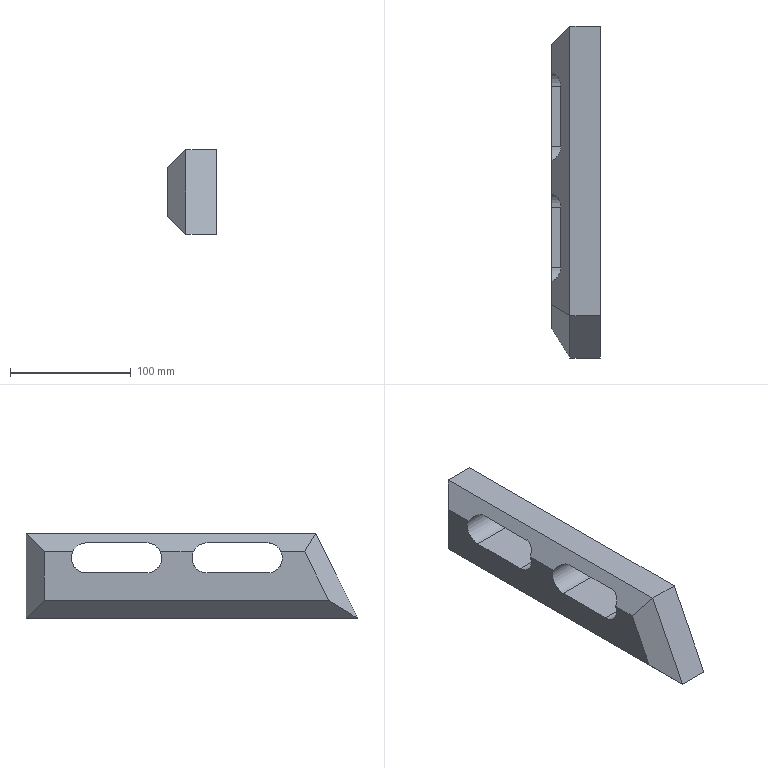Part | SolidWorks | features Chamfer 1, Extrusion 1 | 1 solid | 18 faces | box 40 x 275 x 70 mm | volume 515457 mm3 | plane 14 | cylinder 4 | commonest cylinder face diameters 25 x4
STEP:
#1=CARTESIAN_POINT('',(20.,140.,-7.5));
#2=VERTEX_POINT('',#1);
#3=CARTESIAN_POINT('',(20.,140.,-32.5));
#4=VERTEX_POINT('',#3);
#5=CARTESIAN_POINT('',(20.,140.,-20.));
#6=DIRECTION('',(1.,0.,0.));
#7=DIRECTION('',(0.,0.,-1.));
#8=AXIS2_PLACEMENT_3D('',#5,#6,#7);
#9=CIRCLE('',#8,12.5);
#10=EDGE_CURVE('',#2,#4,#9,.T.);
#11=ORIENTED_EDGE('',*,*,#10,.F.);
#12=CARTESIAN_POINT('',(20.,190.,-7.5));
#13=VERTEX_POINT('',#12);
#14=CARTESIAN_POINT('',(20.,140.,-7.5));
#15=DIRECTION('',(0.,-1.,0.));
#16=VECTOR('',#15,1000.);
#17=LINE('',#14,#16);
#18=EDGE_CURVE('',#13,#2,#17,.T.);
#19=ORIENTED_EDGE('',*,*,#18,.F.);
#20=CARTESIAN_POINT('',(20.,190.,-32.5));
#21=VERTEX_POINT('',#20);
#22=CARTESIAN_POINT('',(20.,190.,-20.));
#23=DIRECTION('',(1.,0.,0.));
#24=DIRECTION('',(0.,0.,-1.));
#25=AXIS2_PLACEMENT_3D('',#22,#23,#24);
#26=CIRCLE('',#25,12.5);
#27=EDGE_CURVE('',#21,#13,#26,.T.);
#28=ORIENTED_EDGE('',*,*,#27,.F.);
#29=CARTESIAN_POINT('',(20.,140.,-32.5));
#30=DIRECTION('',(0.,1.,0.));
#31=VECTOR('',#30,1000.);
#32=LINE('',#29,#31);
#33=EDGE_CURVE('',#4,#21,#32,.T.);
#34=ORIENTED_EDGE('',*,*,#33,.F.);
#35=EDGE_LOOP('',(#11,#19,#28,#34));
#36=FACE_BOUND('',#35,.T.);
#37=CARTESIAN_POINT('',(20.,240.,0.));
#38=VERTEX_POINT('',#37);
#39=CARTESIAN_POINT('',(20.,0.,0.));
#40=VERTEX_POINT('',#39);
#41=CARTESIAN_POINT('',(20.,240.,0.));
#42=DIRECTION('',(0.,-1.,0.));
#43=VECTOR('',#42,1000.);
#44=LINE('',#41,#43);
#45=EDGE_CURVE('',#38,#40,#44,.T.);
#46=ORIENTED_EDGE('',*,*,#45,.T.);
#47=CARTESIAN_POINT('',(20.,-35.,-70.));
#48=VERTEX_POINT('',#47);
#49=CARTESIAN_POINT('',(20.,0.,0.));
#50=DIRECTION('',(0.,-0.4472,-0.8944));
#51=VECTOR('',#50,1000.);
#52=LINE('',#49,#51);
#53=EDGE_CURVE('',#40,#48,#52,.T.);
#54=ORIENTED_EDGE('',*,*,#53,.T.);
#55=CARTESIAN_POINT('',(20.,240.,-70.));
#56=VERTEX_POINT('',#55);
#57=CARTESIAN_POINT('',(20.,-35.,-70.));
#58=DIRECTION('',(0.,1.,0.));
#59=VECTOR('',#58,1000.);
#60=LINE('',#57,#59);
#61=EDGE_CURVE('',#48,#56,#60,.T.);
#62=ORIENTED_EDGE('',*,*,#61,.T.);
#63=CARTESIAN_POINT('',(20.,240.,-70.));
#64=DIRECTION('',(0.,0.,1.));
#65=VECTOR('',#64,1000.);
#66=LINE('',#63,#65);
#67=EDGE_CURVE('',#56,#38,#66,.T.);
#68=ORIENTED_EDGE('',*,*,#67,.T.);
#69=EDGE_LOOP('',(#46,#54,#62,#68));
#70=FACE_OUTER_BOUND('',#69,.T.);
#71=CARTESIAN_POINT('',(20.,40.,-7.5));
#72=VERTEX_POINT('',#71);
#73=CARTESIAN_POINT('',(20.,40.,-32.5));
#74=VERTEX_POINT('',#73);
#75=CARTESIAN_POINT('',(20.,40.,-20.));
#76=DIRECTION('',(1.,0.,0.));
#77=DIRECTION('',(0.,0.,-1.));
#78=AXIS2_PLACEMENT_3D('',#75,#76,#77);
#79=CIRCLE('',#78,12.5);
#80=EDGE_CURVE('',#72,#74,#79,.T.);
#81=ORIENTED_EDGE('',*,*,#80,.F.);
#82=CARTESIAN_POINT('',(20.,90.,-7.5));
#83=VERTEX_POINT('',#82);
#84=CARTESIAN_POINT('',(20.,40.,-7.5));
#85=DIRECTION('',(0.,-1.,0.));
#86=VECTOR('',#85,1000.);
#87=LINE('',#84,#86);
#88=EDGE_CURVE('',#83,#72,#87,.T.);
#89=ORIENTED_EDGE('',*,*,#88,.F.);
#90=CARTESIAN_POINT('',(20.,90.,-32.5));
#91=VERTEX_POINT('',#90);
#92=CARTESIAN_POINT('',(20.,90.,-20.));
#93=DIRECTION('',(1.,0.,0.));
#94=DIRECTION('',(0.,0.,-1.));
#95=AXIS2_PLACEMENT_3D('',#92,#93,#94);
#96=CIRCLE('',#95,12.5);
#97=EDGE_CURVE('',#91,#83,#96,.T.);
#98=ORIENTED_EDGE('',*,*,#97,.F.);
#99=CARTESIAN_POINT('',(20.,40.,-32.5));
#100=DIRECTION('',(0.,1.,0.));
#101=VECTOR('',#100,1000.);
#102=LINE('',#99,#101);
#103=EDGE_CURVE('',#74,#91,#102,.T.);
#104=ORIENTED_EDGE('',*,*,#103,.F.);
#105=EDGE_LOOP('',(#81,#89,#98,#104));
#106=FACE_BOUND('',#105,.T.);
#107=CARTESIAN_POINT('',(20.,0.,0.));
#108=DIRECTION('',(-1.,0.,0.));
#109=DIRECTION('',(0.,0.,1.));
#110=AXIS2_PLACEMENT_3D('',#107,#108,#109);
#111=PLANE('',#110);
#112=ADVANCED_FACE('',(#36,#70,#106),#111,.F.);
#113=CARTESIAN_POINT('',(-20.,90.,-32.5));
#114=VERTEX_POINT('',#113);
#115=CARTESIAN_POINT('',(-20.,101.456,-15.));
#116=VERTEX_POINT('',#115);
#117=CARTESIAN_POINT('',(-20.,90.,-20.));
#118=DIRECTION('',(1.,0.,0.));
#119=DIRECTION('',(0.,0.,-1.));
#120=AXIS2_PLACEMENT_3D('',#117,#118,#119);
#121=CIRCLE('',#120,12.5);
#122=EDGE_CURVE('',#114,#116,#121,.T.);
#123=ORIENTED_EDGE('',*,*,#122,.T.);
#124=CARTESIAN_POINT('',(-20.,128.544,-15.));
#125=VERTEX_POINT('',#124);
#126=CARTESIAN_POINT('',(-20.,240.,-15.));
#127=DIRECTION('',(0.,1.,0.));
#128=VECTOR('',#127,1000.);
#129=LINE('',#126,#128);
#130=EDGE_CURVE('',#116,#125,#129,.T.);
#131=ORIENTED_EDGE('',*,*,#130,.T.);
#132=CARTESIAN_POINT('',(-20.,140.,-32.5));
#133=VERTEX_POINT('',#132);
#134=CARTESIAN_POINT('',(-20.,140.,-20.));
#135=DIRECTION('',(1.,0.,0.));
#136=DIRECTION('',(0.,0.,-1.));
#137=AXIS2_PLACEMENT_3D('',#134,#135,#136);
#138=CIRCLE('',#137,12.5);
#139=EDGE_CURVE('',#125,#133,#138,.T.);
#140=ORIENTED_EDGE('',*,*,#139,.T.);
#141=CARTESIAN_POINT('',(-20.,190.,-32.5));
#142=VERTEX_POINT('',#141);
#143=CARTESIAN_POINT('',(-20.,140.,-32.5));
#144=DIRECTION('',(0.,1.,0.));
#145=VECTOR('',#144,1000.);
#146=LINE('',#143,#145);
#147=EDGE_CURVE('',#133,#142,#146,.T.);
#148=ORIENTED_EDGE('',*,*,#147,.T.);
#149=CARTESIAN_POINT('',(-20.,201.456,-15.));
#150=VERTEX_POINT('',#149);
#151=CARTESIAN_POINT('',(-20.,190.,-20.));
#152=DIRECTION('',(1.,0.,0.));
#153=DIRECTION('',(0.,0.,-1.));
#154=AXIS2_PLACEMENT_3D('',#151,#152,#153);
#155=CIRCLE('',#154,12.5);
#156=EDGE_CURVE('',#142,#150,#155,.T.);
#157=ORIENTED_EDGE('',*,*,#156,.T.);
#158=CARTESIAN_POINT('',(-20.,225.,-15.));
#159=VERTEX_POINT('',#158);
#160=CARTESIAN_POINT('',(-20.,240.,-15.));
#161=DIRECTION('',(0.,1.,0.));
#162=VECTOR('',#161,1000.);
#163=LINE('',#160,#162);
#164=EDGE_CURVE('',#150,#159,#163,.T.);
#165=ORIENTED_EDGE('',*,*,#164,.T.);
#166=CARTESIAN_POINT('',(-20.,225.,-55.));
#167=VERTEX_POINT('',#166);
#168=CARTESIAN_POINT('',(-20.,225.,-70.));
#169=DIRECTION('',(0.,0.,-1.));
#170=VECTOR('',#169,1000.);
#171=LINE('',#168,#170);
#172=EDGE_CURVE('',#159,#167,#171,.T.);
#173=ORIENTED_EDGE('',*,*,#172,.T.);
#174=CARTESIAN_POINT('',(-20.,-10.729,-55.));
#175=VERTEX_POINT('',#174);
#176=CARTESIAN_POINT('',(-20.,-35.,-55.));
#177=DIRECTION('',(0.,-1.,0.));
#178=VECTOR('',#177,1000.);
#179=LINE('',#176,#178);
#180=EDGE_CURVE('',#167,#175,#179,.T.);
#181=ORIENTED_EDGE('',*,*,#180,.T.);
#182=CARTESIAN_POINT('',(-20.,9.271,-15.));
#183=VERTEX_POINT('',#182);
#184=CARTESIAN_POINT('',(-20.,13.416,-6.708));
#185=DIRECTION('',(0.,0.4472,0.8944));
#186=VECTOR('',#185,1000.);
#187=LINE('',#184,#186);
#188=EDGE_CURVE('',#175,#183,#187,.T.);
#189=ORIENTED_EDGE('',*,*,#188,.T.);
#190=CARTESIAN_POINT('',(-20.,28.544,-15.));
#191=VERTEX_POINT('',#190);
#192=CARTESIAN_POINT('',(-20.,240.,-15.));
#193=DIRECTION('',(0.,1.,0.));
#194=VECTOR('',#193,1000.);
#195=LINE('',#192,#194);
#196=EDGE_CURVE('',#183,#191,#195,.T.);
#197=ORIENTED_EDGE('',*,*,#196,.T.);
#198=CARTESIAN_POINT('',(-20.,40.,-32.5));
#199=VERTEX_POINT('',#198);
#200=CARTESIAN_POINT('',(-20.,40.,-20.));
#201=DIRECTION('',(1.,0.,0.));
#202=DIRECTION('',(0.,0.,-1.));
#203=AXIS2_PLACEMENT_3D('',#200,#201,#202);
#204=CIRCLE('',#203,12.5);
#205=EDGE_CURVE('',#191,#199,#204,.T.);
#206=ORIENTED_EDGE('',*,*,#205,.T.);
#207=CARTESIAN_POINT('',(-20.,40.,-32.5));
#208=DIRECTION('',(0.,1.,0.));
#209=VECTOR('',#208,1000.);
#210=LINE('',#207,#209);
#211=EDGE_CURVE('',#199,#114,#210,.T.);
#212=ORIENTED_EDGE('',*,*,#211,.T.);
#213=EDGE_LOOP('',(#123,#131,#140,#148,#157,#165,#173,#181,#189,#197,#206,#212));
#214=FACE_OUTER_BOUND('',#213,.T.);
#215=CARTESIAN_POINT('',(-20.,0.,0.));
#216=DIRECTION('',(-1.,0.,0.));
#217=DIRECTION('',(0.,0.,1.));
#218=AXIS2_PLACEMENT_3D('',#215,#216,#217);
#219=PLANE('',#218);
#220=ADVANCED_FACE('',(#214),#219,.T.);
#221=CARTESIAN_POINT('',(-5.,240.,0.));
#222=VERTEX_POINT('',#221);
#223=CARTESIAN_POINT('',(20.,240.,0.));
#224=DIRECTION('',(-1.,0.,0.));
#225=VECTOR('',#224,1000.);
#226=LINE('',#223,#225);
#227=EDGE_CURVE('',#38,#222,#226,.T.);
#228=ORIENTED_EDGE('',*,*,#227,.T.);
#229=CARTESIAN_POINT('',(-5.,0.,0.));
#230=VERTEX_POINT('',#229);
#231=CARTESIAN_POINT('',(-5.,0.,0.));
#232=DIRECTION('',(0.,-1.,0.));
#233=VECTOR('',#232,1000.);
#234=LINE('',#231,#233);
#235=EDGE_CURVE('',#222,#230,#234,.T.);
#236=ORIENTED_EDGE('',*,*,#235,.T.);
#237=CARTESIAN_POINT('',(20.,0.,0.));
#238=DIRECTION('',(-1.,0.,0.));
#239=VECTOR('',#238,1000.);
#240=LINE('',#237,#239);
#241=EDGE_CURVE('',#40,#230,#240,.T.);
#242=ORIENTED_EDGE('',*,*,#241,.F.);
#243=ORIENTED_EDGE('',*,*,#45,.F.);
#244=EDGE_LOOP('',(#228,#236,#242,#243));
#245=FACE_OUTER_BOUND('',#244,.T.);
#246=CARTESIAN_POINT('',(20.,240.,0.));
#247=DIRECTION('',(0.,0.,-1.));
#248=DIRECTION('',(-1.,0.,0.));
#249=AXIS2_PLACEMENT_3D('',#246,#247,#248);
#250=PLANE('',#249);
#251=ADVANCED_FACE('',(#245),#250,.F.);
#252=ORIENTED_EDGE('',*,*,#241,.T.);
#253=CARTESIAN_POINT('',(-5.,-35.,-70.));
#254=VERTEX_POINT('',#253);
#255=CARTESIAN_POINT('',(-5.,-35.,-70.));
#256=DIRECTION('',(0.,-0.4472,-0.8944));
#257=VECTOR('',#256,1000.);
#258=LINE('',#255,#257);
#259=EDGE_CURVE('',#230,#254,#258,.T.);
#260=ORIENTED_EDGE('',*,*,#259,.T.);
#261=CARTESIAN_POINT('',(20.,-35.,-70.));
#262=DIRECTION('',(-1.,0.,0.));
#263=VECTOR('',#262,1000.);
#264=LINE('',#261,#263);
#265=EDGE_CURVE('',#48,#254,#264,.T.);
#266=ORIENTED_EDGE('',*,*,#265,.F.);
#267=ORIENTED_EDGE('',*,*,#53,.F.);
#268=EDGE_LOOP('',(#252,#260,#266,#267));
#269=FACE_OUTER_BOUND('',#268,.T.);
#270=CARTESIAN_POINT('',(20.,0.,0.));
#271=DIRECTION('',(0.,0.8944,-0.4472));
#272=DIRECTION('',(0.,0.4472,0.8944));
#273=AXIS2_PLACEMENT_3D('',#270,#271,#272);
#274=PLANE('',#273);
#275=ADVANCED_FACE('',(#269),#274,.F.);
#276=ORIENTED_EDGE('',*,*,#265,.T.);
#277=CARTESIAN_POINT('',(-5.,240.,-70.));
#278=VERTEX_POINT('',#277);
#279=CARTESIAN_POINT('',(-5.,240.,-70.));
#280=DIRECTION('',(0.,1.,0.));
#281=VECTOR('',#280,1000.);
#282=LINE('',#279,#281);
#283=EDGE_CURVE('',#254,#278,#282,.T.);
#284=ORIENTED_EDGE('',*,*,#283,.T.);
#285=CARTESIAN_POINT('',(20.,240.,-70.));
#286=DIRECTION('',(-1.,0.,0.));
#287=VECTOR('',#286,1000.);
#288=LINE('',#285,#287);
#289=EDGE_CURVE('',#56,#278,#288,.T.);
#290=ORIENTED_EDGE('',*,*,#289,.F.);
#291=ORIENTED_EDGE('',*,*,#61,.F.);
#292=EDGE_LOOP('',(#276,#284,#290,#291));
#293=FACE_OUTER_BOUND('',#292,.T.);
#294=CARTESIAN_POINT('',(20.,-35.,-70.));
#295=DIRECTION('',(0.,0.,1.));
#296=DIRECTION('',(0.,-1.,0.));
#297=AXIS2_PLACEMENT_3D('',#294,#295,#296);
#298=PLANE('',#297);
#299=ADVANCED_FACE('',(#293),#298,.F.);
#300=ORIENTED_EDGE('',*,*,#289,.T.);
#301=CARTESIAN_POINT('',(-5.,240.,0.));
#302=DIRECTION('',(0.,0.,1.));
#303=VECTOR('',#302,1000.);
#304=LINE('',#301,#303);
#305=EDGE_CURVE('',#278,#222,#304,.T.);
#306=ORIENTED_EDGE('',*,*,#305,.T.);
#307=ORIENTED_EDGE('',*,*,#227,.F.);
#308=ORIENTED_EDGE('',*,*,#67,.F.);
#309=EDGE_LOOP('',(#300,#306,#307,#308));
#310=FACE_OUTER_BOUND('',#309,.T.);
#311=CARTESIAN_POINT('',(20.,240.,-70.));
#312=DIRECTION('',(0.,-1.,0.));
#313=DIRECTION('',(0.,0.,-1.));
#314=AXIS2_PLACEMENT_3D('',#311,#312,#313);
#315=PLANE('',#314);
#316=ADVANCED_FACE('',(#310),#315,.F.);
#317=ORIENTED_EDGE('',*,*,#139,.F.);
#318=CARTESIAN_POINT('',(-12.5,140.,-7.5));
#319=VERTEX_POINT('',#318);
#320=CARTESIAN_POINT('',(-20.,128.544,-15.));
#321=CARTESIAN_POINT('',(-15.306,130.592,-10.306));
#322=CARTESIAN_POINT('',(-12.5,134.878,-7.5));
#323=CARTESIAN_POINT('',(-12.5,140.,-7.5));
#324=(BOUNDED_CURVE()B_SPLINE_CURVE(3,(#320,#321,#322,#323),.UNSPECIFIED.,.F.,.T.)B_SPLINE_CURVE_WITH_KNOTS((4,4),(1.982,3.142),.UNSPECIFIED.)CURVE()GEOMETRIC_REPRESENTATION_ITEM()RATIONAL_B_SPLINE_CURVE((1.,0.8911,0.8911,1.))REPRESENTATION_ITEM(''));
#325=EDGE_CURVE('',#125,#319,#324,.T.);
#326=ORIENTED_EDGE('',*,*,#325,.T.);
#327=CARTESIAN_POINT('',(20.,140.,-7.5));
#328=DIRECTION('',(-1.,0.,0.));
#329=VECTOR('',#328,1000.);
#330=LINE('',#327,#329);
#331=EDGE_CURVE('',#2,#319,#330,.T.);
#332=ORIENTED_EDGE('',*,*,#331,.F.);
#333=ORIENTED_EDGE('',*,*,#10,.T.);
#334=CARTESIAN_POINT('',(20.,140.,-32.5));
#335=DIRECTION('',(-1.,0.,0.));
#336=VECTOR('',#335,1000.);
#337=LINE('',#334,#336);
#338=EDGE_CURVE('',#4,#133,#337,.T.);
#339=ORIENTED_EDGE('',*,*,#338,.T.);
#340=EDGE_LOOP('',(#317,#326,#332,#333,#339));
#341=FACE_OUTER_BOUND('',#340,.T.);
#342=CARTESIAN_POINT('',(20.,140.,-20.));
#343=DIRECTION('',(-1.,0.,0.));
#344=DIRECTION('',(0.,0.,1.));
#345=AXIS2_PLACEMENT_3D('',#342,#343,#344);
#346=CYLINDRICAL_SURFACE('',#345,12.5);
#347=ADVANCED_FACE('',(#341),#346,.F.);
#348=ORIENTED_EDGE('',*,*,#147,.F.);
#349=ORIENTED_EDGE('',*,*,#338,.F.);
#350=ORIENTED_EDGE('',*,*,#33,.T.);
#351=CARTESIAN_POINT('',(20.,190.,-32.5));
#352=DIRECTION('',(-1.,0.,0.));
#353=VECTOR('',#352,1000.);
#354=LINE('',#351,#353);
#355=EDGE_CURVE('',#21,#142,#354,.T.);
#356=ORIENTED_EDGE('',*,*,#355,.T.);
#357=EDGE_LOOP('',(#348,#349,#350,#356));
#358=FACE_OUTER_BOUND('',#357,.T.);
#359=CARTESIAN_POINT('',(20.,140.,-32.5));
#360=DIRECTION('',(0.,0.,1.));
#361=DIRECTION('',(1.,0.,0.));
#362=AXIS2_PLACEMENT_3D('',#359,#360,#361);
#363=PLANE('',#362);
#364=ADVANCED_FACE('',(#358),#363,.T.);
#365=CARTESIAN_POINT('',(-12.5,190.,-7.5));
#366=VERTEX_POINT('',#365);
#367=CARTESIAN_POINT('',(20.,190.,-7.5));
#368=DIRECTION('',(-1.,0.,0.));
#369=VECTOR('',#368,1000.);
#370=LINE('',#367,#369);
#371=EDGE_CURVE('',#13,#366,#370,.T.);
#372=ORIENTED_EDGE('',*,*,#371,.T.);
#373=CARTESIAN_POINT('',(-12.5,190.,-7.5));
#374=CARTESIAN_POINT('',(-12.5,195.122,-7.5));
#375=CARTESIAN_POINT('',(-15.306,199.408,-10.306));
#376=CARTESIAN_POINT('',(-20.,201.456,-15.));
#377=(BOUNDED_CURVE()B_SPLINE_CURVE(3,(#373,#374,#375,#376),.UNSPECIFIED.,.F.,.T.)B_SPLINE_CURVE_WITH_KNOTS((4,4),(3.142,4.301),.UNSPECIFIED.)CURVE()GEOMETRIC_REPRESENTATION_ITEM()RATIONAL_B_SPLINE_CURVE((1.,0.8911,0.8911,1.))REPRESENTATION_ITEM(''));
#378=EDGE_CURVE('',#366,#150,#377,.T.);
#379=ORIENTED_EDGE('',*,*,#378,.T.);
#380=ORIENTED_EDGE('',*,*,#156,.F.);
#381=ORIENTED_EDGE('',*,*,#355,.F.);
#382=ORIENTED_EDGE('',*,*,#27,.T.);
#383=EDGE_LOOP('',(#372,#379,#380,#381,#382));
#384=FACE_OUTER_BOUND('',#383,.T.);
#385=CARTESIAN_POINT('',(20.,190.,-20.));
#386=DIRECTION('',(-1.,0.,0.));
#387=DIRECTION('',(0.,0.,1.));
#388=AXIS2_PLACEMENT_3D('',#385,#386,#387);
#389=CYLINDRICAL_SURFACE('',#388,12.5);
#390=ADVANCED_FACE('',(#384),#389,.F.);
#391=ORIENTED_EDGE('',*,*,#331,.T.);
#392=CARTESIAN_POINT('',(-12.5,140.,-7.5));
#393=DIRECTION('',(0.,1.,0.));
#394=VECTOR('',#393,1000.);
#395=LINE('',#392,#394);
#396=EDGE_CURVE('',#319,#366,#395,.T.);
#397=ORIENTED_EDGE('',*,*,#396,.T.);
#398=ORIENTED_EDGE('',*,*,#371,.F.);
#399=ORIENTED_EDGE('',*,*,#18,.T.);
#400=EDGE_LOOP('',(#391,#397,#398,#399));
#401=FACE_OUTER_BOUND('',#400,.T.);
#402=CARTESIAN_POINT('',(20.,140.,-7.5));
#403=DIRECTION('',(0.,0.,-1.));
#404=DIRECTION('',(-1.,0.,0.));
#405=AXIS2_PLACEMENT_3D('',#402,#403,#404);
#406=PLANE('',#405);
#407=ADVANCED_FACE('',(#401),#406,.T.);
#408=ORIENTED_EDGE('',*,*,#205,.F.);
#409=CARTESIAN_POINT('',(-12.5,40.,-7.5));
#410=VERTEX_POINT('',#409);
#411=CARTESIAN_POINT('',(-20.,28.544,-15.));
#412=CARTESIAN_POINT('',(-15.306,30.592,-10.306));
#413=CARTESIAN_POINT('',(-12.5,34.878,-7.5));
#414=CARTESIAN_POINT('',(-12.5,40.,-7.5));
#415=(BOUNDED_CURVE()B_SPLINE_CURVE(3,(#411,#412,#413,#414),.UNSPECIFIED.,.F.,.T.)B_SPLINE_CURVE_WITH_KNOTS((4,4),(1.982,3.142),.UNSPECIFIED.)CURVE()GEOMETRIC_REPRESENTATION_ITEM()RATIONAL_B_SPLINE_CURVE((1.,0.8911,0.8911,1.))REPRESENTATION_ITEM(''));
#416=EDGE_CURVE('',#191,#410,#415,.T.);
#417=ORIENTED_EDGE('',*,*,#416,.T.);
#418=CARTESIAN_POINT('',(20.,40.,-7.5));
#419=DIRECTION('',(-1.,0.,0.));
#420=VECTOR('',#419,1000.);
#421=LINE('',#418,#420);
#422=EDGE_CURVE('',#72,#410,#421,.T.);
#423=ORIENTED_EDGE('',*,*,#422,.F.);
#424=ORIENTED_EDGE('',*,*,#80,.T.);
#425=CARTESIAN_POINT('',(20.,40.,-32.5));
#426=DIRECTION('',(-1.,0.,0.));
#427=VECTOR('',#426,1000.);
#428=LINE('',#425,#427);
#429=EDGE_CURVE('',#74,#199,#428,.T.);
#430=ORIENTED_EDGE('',*,*,#429,.T.);
#431=EDGE_LOOP('',(#408,#417,#423,#424,#430));
#432=FACE_OUTER_BOUND('',#431,.T.);
#433=CARTESIAN_POINT('',(20.,40.,-20.));
#434=DIRECTION('',(-1.,0.,0.));
#435=DIRECTION('',(0.,0.,1.));
#436=AXIS2_PLACEMENT_3D('',#433,#434,#435);
#437=CYLINDRICAL_SURFACE('',#436,12.5);
#438=ADVANCED_FACE('',(#432),#437,.F.);
#439=ORIENTED_EDGE('',*,*,#211,.F.);
#440=ORIENTED_EDGE('',*,*,#429,.F.);
#441=ORIENTED_EDGE('',*,*,#103,.T.);
#442=CARTESIAN_POINT('',(20.,90.,-32.5));
#443=DIRECTION('',(-1.,0.,0.));
#444=VECTOR('',#443,1000.);
#445=LINE('',#442,#444);
#446=EDGE_CURVE('',#91,#114,#445,.T.);
#447=ORIENTED_EDGE('',*,*,#446,.T.);
#448=EDGE_LOOP('',(#439,#440,#441,#447));
#449=FACE_OUTER_BOUND('',#448,.T.);
#450=CARTESIAN_POINT('',(20.,40.,-32.5));
#451=DIRECTION('',(0.,0.,1.));
#452=DIRECTION('',(1.,0.,0.));
#453=AXIS2_PLACEMENT_3D('',#450,#451,#452);
#454=PLANE('',#453);
#455=ADVANCED_FACE('',(#449),#454,.T.);
#456=CARTESIAN_POINT('',(-12.5,90.,-7.5));
#457=VERTEX_POINT('',#456);
#458=CARTESIAN_POINT('',(20.,90.,-7.5));
#459=DIRECTION('',(-1.,0.,0.));
#460=VECTOR('',#459,1000.);
#461=LINE('',#458,#460);
#462=EDGE_CURVE('',#83,#457,#461,.T.);
#463=ORIENTED_EDGE('',*,*,#462,.T.);
#464=CARTESIAN_POINT('',(-12.5,90.,-7.5));
#465=CARTESIAN_POINT('',(-12.5,95.122,-7.5));
#466=CARTESIAN_POINT('',(-15.306,99.408,-10.306));
#467=CARTESIAN_POINT('',(-20.,101.456,-15.));
#468=(BOUNDED_CURVE()B_SPLINE_CURVE(3,(#464,#465,#466,#467),.UNSPECIFIED.,.F.,.F.)B_SPLINE_CURVE_WITH_KNOTS((4,4),(3.142,4.301),.UNSPECIFIED.)CURVE()GEOMETRIC_REPRESENTATION_ITEM()RATIONAL_B_SPLINE_CURVE((1.,0.8911,0.8911,1.))REPRESENTATION_ITEM(''));
#469=EDGE_CURVE('',#457,#116,#468,.T.);
#470=ORIENTED_EDGE('',*,*,#469,.T.);
#471=ORIENTED_EDGE('',*,*,#122,.F.);
#472=ORIENTED_EDGE('',*,*,#446,.F.);
#473=ORIENTED_EDGE('',*,*,#97,.T.);
#474=EDGE_LOOP('',(#463,#470,#471,#472,#473));
#475=FACE_OUTER_BOUND('',#474,.T.);
#476=CARTESIAN_POINT('',(20.,90.,-20.));
#477=DIRECTION('',(-1.,0.,0.));
#478=DIRECTION('',(0.,0.,1.));
#479=AXIS2_PLACEMENT_3D('',#476,#477,#478);
#480=CYLINDRICAL_SURFACE('',#479,12.5);
#481=ADVANCED_FACE('',(#475),#480,.F.);
#482=ORIENTED_EDGE('',*,*,#422,.T.);
#483=CARTESIAN_POINT('',(-12.5,40.,-7.5));
#484=DIRECTION('',(0.,1.,0.));
#485=VECTOR('',#484,1000.);
#486=LINE('',#483,#485);
#487=EDGE_CURVE('',#410,#457,#486,.T.);
#488=ORIENTED_EDGE('',*,*,#487,.T.);
#489=ORIENTED_EDGE('',*,*,#462,.F.);
#490=ORIENTED_EDGE('',*,*,#88,.T.);
#491=EDGE_LOOP('',(#482,#488,#489,#490));
#492=FACE_OUTER_BOUND('',#491,.T.);
#493=CARTESIAN_POINT('',(20.,40.,-7.5));
#494=DIRECTION('',(0.,0.,-1.));
#495=DIRECTION('',(-1.,0.,0.));
#496=AXIS2_PLACEMENT_3D('',#493,#494,#495);
#497=PLANE('',#496);
#498=ADVANCED_FACE('',(#492),#497,.T.);
#499=CARTESIAN_POINT('',(-5.,240.,-70.));
#500=DIRECTION('',(0.5774,0.5774,-0.5774));
#501=VECTOR('',#500,1000.);
#502=LINE('',#499,#501);
#503=EDGE_CURVE('',#167,#278,#502,.T.);
#504=ORIENTED_EDGE('',*,*,#503,.F.);
#505=ORIENTED_EDGE('',*,*,#172,.F.);
#506=CARTESIAN_POINT('',(-28.333,216.667,-23.333));
#507=DIRECTION('',(-0.5774,-0.5774,-0.5774));
#508=VECTOR('',#507,1000.);
#509=LINE('',#506,#508);
#510=EDGE_CURVE('',#222,#159,#509,.T.);
#511=ORIENTED_EDGE('',*,*,#510,.F.);
#512=ORIENTED_EDGE('',*,*,#305,.F.);
#513=EDGE_LOOP('',(#504,#505,#511,#512));
#514=FACE_OUTER_BOUND('',#513,.T.);
#515=CARTESIAN_POINT('',(-5.,240.,-70.));
#516=DIRECTION('',(-0.7071,0.7071,0.));
#517=DIRECTION('',(0.,0.,-1.));
#518=AXIS2_PLACEMENT_3D('',#515,#516,#517);
#519=PLANE('',#518);
#520=ADVANCED_FACE('',(#514),#519,.T.);
#521=ORIENTED_EDGE('',*,*,#416,.F.);
#522=ORIENTED_EDGE('',*,*,#196,.F.);
#523=CARTESIAN_POINT('',(-67.271,38.486,-62.271));
#524=DIRECTION('',(-0.6479,0.4004,-0.6479));
#525=VECTOR('',#524,1000.);
#526=LINE('',#523,#525);
#527=EDGE_CURVE('',#230,#183,#526,.T.);
#528=ORIENTED_EDGE('',*,*,#527,.F.);
#529=ORIENTED_EDGE('',*,*,#235,.F.);
#530=ORIENTED_EDGE('',*,*,#510,.T.);
#531=ORIENTED_EDGE('',*,*,#164,.F.);
#532=ORIENTED_EDGE('',*,*,#378,.F.);
#533=ORIENTED_EDGE('',*,*,#396,.F.);
#534=ORIENTED_EDGE('',*,*,#325,.F.);
#535=ORIENTED_EDGE('',*,*,#130,.F.);
#536=ORIENTED_EDGE('',*,*,#469,.F.);
#537=ORIENTED_EDGE('',*,*,#487,.F.);
#538=EDGE_LOOP('',(#521,#522,#528,#529,#530,#531,#532,#533,#534,#535,#536,#537));
#539=FACE_OUTER_BOUND('',#538,.T.);
#540=CARTESIAN_POINT('',(-5.,240.,0.));
#541=DIRECTION('',(-0.7071,0.,0.7071));
#542=DIRECTION('',(0.,1.,0.));
#543=AXIS2_PLACEMENT_3D('',#540,#541,#542);
#544=PLANE('',#543);
#545=ADVANCED_FACE('',(#539),#544,.T.);
#546=ORIENTED_EDGE('',*,*,#503,.T.);
#547=ORIENTED_EDGE('',*,*,#283,.F.);
#548=CARTESIAN_POINT('',(-5.,-35.,-70.));
#549=DIRECTION('',(0.4653,-0.7529,-0.4653));
#550=VECTOR('',#549,1000.);
#551=LINE('',#548,#550);
#552=EDGE_CURVE('',#175,#254,#551,.T.);
#553=ORIENTED_EDGE('',*,*,#552,.F.);
#554=ORIENTED_EDGE('',*,*,#180,.F.);
#555=EDGE_LOOP('',(#546,#547,#553,#554));
#556=FACE_OUTER_BOUND('',#555,.T.);
#557=CARTESIAN_POINT('',(-5.,-35.,-70.));
#558=DIRECTION('',(-0.7071,0.,-0.7071));
#559=DIRECTION('',(0.,-1.,0.));
#560=AXIS2_PLACEMENT_3D('',#557,#558,#559);
#561=PLANE('',#560);
#562=ADVANCED_FACE('',(#556),#561,.T.);
#563=ORIENTED_EDGE('',*,*,#527,.T.);
#564=ORIENTED_EDGE('',*,*,#188,.F.);
#565=ORIENTED_EDGE('',*,*,#552,.T.);
#566=ORIENTED_EDGE('',*,*,#259,.F.);
#567=EDGE_LOOP('',(#563,#564,#565,#566));
#568=FACE_OUTER_BOUND('',#567,.T.);
#569=CARTESIAN_POINT('',(-5.,0.,0.));
#570=DIRECTION('',(-0.7071,-0.6325,0.3162));
#571=DIRECTION('',(0.,0.4472,0.8944));
#572=AXIS2_PLACEMENT_3D('',#569,#570,#571);
#573=PLANE('',#572);
#574=ADVANCED_FACE('',(#568),#573,.T.);
#575=CLOSED_SHELL('',(#112,#220,#251,#275,#299,#316,#347,#364,#390,#407,#438,#455,#481,#498,#520,#545,#562,#574));
#576=MANIFOLD_SOLID_BREP('',#575);
#577=CARTESIAN_POINT('',(0.,0.,0.));
#578=DIRECTION('',(0.,0.,1.));
#579=DIRECTION('',(1.,0.,0.));
#580=AXIS2_PLACEMENT_3D('',#577,#578,#579);
#581=(LENGTH_UNIT()NAMED_UNIT(*)SI_UNIT(.MILLI.,.METRE.));
#582=UNCERTAINTY_MEASURE_WITH_UNIT(LENGTH_MEASURE(0.00001),#581,'','');
#583=(NAMED_UNIT(*)PLANE_ANGLE_UNIT()SI_UNIT($,.RADIAN.));
#584=(NAMED_UNIT(*)SI_UNIT($,.STERADIAN.)SOLID_ANGLE_UNIT());
#585=(GEOMETRIC_REPRESENTATION_CONTEXT(3)GLOBAL_UNCERTAINTY_ASSIGNED_CONTEXT((#582))GLOBAL_UNIT_ASSIGNED_CONTEXT((#581,#583,#584))REPRESENTATION_CONTEXT('',''));
#586=ADVANCED_BREP_SHAPE_REPRESENTATION('',(#576,#580),#585);